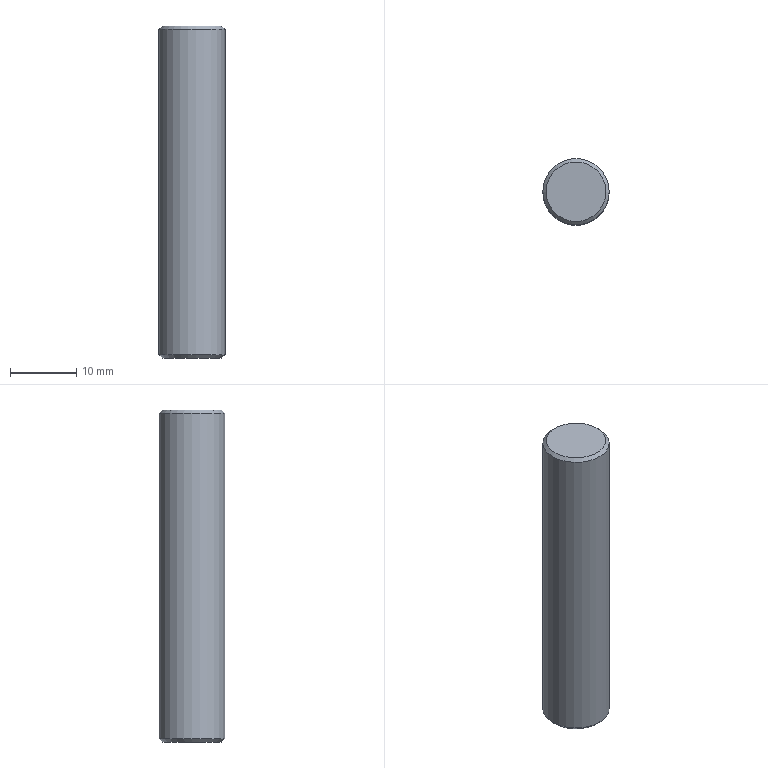Part | STEP file | D8-50_id50_x_t | 1 solid | 5 faces | box 10 x 10 x 50 mm | volume 3919 mm3 | plane 2 | cone 2 | cylinder 1 | commonest cylinder face diameters 10 x1
STEP:
#1=CARTESIAN_POINT('',(-224.05,-48.,-64.5));
#2=VERTEX_POINT('',#1);
#3=CARTESIAN_POINT('',(-219.55,-48.,-64.5));
#4=DIRECTION('',(0.,0.,-1.));
#5=DIRECTION('',(-1.,0.,0.));
#6=AXIS2_PLACEMENT_3D('',#3,#4,#5);
#7=CIRCLE('',#6,4.5);
#8=EDGE_CURVE('',#2,#2,#7,.T.);
#9=ORIENTED_EDGE('',*,*,#8,.T.);
#10=EDGE_LOOP('',(#9));
#11=FACE_OUTER_BOUND('',#10,.T.);
#12=CARTESIAN_POINT('',(-219.55,-48.,-64.5));
#13=DIRECTION('',(0.,0.,-1.));
#14=DIRECTION('',(-1.,0.,0.));
#15=AXIS2_PLACEMENT_3D('',#12,#13,#14);
#16=PLANE('',#15);
#17=ADVANCED_FACE('',(#11),#16,.T.);
#18=CARTESIAN_POINT('',(-224.55,-48.,-64.));
#19=VERTEX_POINT('',#18);
#20=CARTESIAN_POINT('',(-219.55,-48.,-64.));
#21=DIRECTION('',(0.,0.,1.));
#22=DIRECTION('',(-1.,0.,0.));
#23=AXIS2_PLACEMENT_3D('',#20,#21,#22);
#24=CIRCLE('',#23,5.);
#25=EDGE_CURVE('',#19,#19,#24,.T.);
#26=ORIENTED_EDGE('',*,*,#25,.T.);
#27=EDGE_LOOP('',(#26));
#28=FACE_BOUND('',#27,.T.);
#29=CARTESIAN_POINT('',(-214.55,-48.,-15.));
#30=VERTEX_POINT('',#29);
#31=CARTESIAN_POINT('',(-219.55,-48.,-15.));
#32=DIRECTION('',(0.,0.,-1.));
#33=DIRECTION('',(1.,0.,0.));
#34=AXIS2_PLACEMENT_3D('',#31,#32,#33);
#35=CIRCLE('',#34,5.);
#36=EDGE_CURVE('',#30,#30,#35,.T.);
#37=ORIENTED_EDGE('',*,*,#36,.T.);
#38=EDGE_LOOP('',(#37));
#39=FACE_BOUND('',#38,.T.);
#40=CARTESIAN_POINT('',(-219.55,-48.,-47.));
#41=DIRECTION('',(0.,0.,-1.));
#42=DIRECTION('',(1.,0.,0.));
#43=AXIS2_PLACEMENT_3D('',#40,#41,#42);
#44=CYLINDRICAL_SURFACE('',#43,5.);
#45=ADVANCED_FACE('',(#28,#39),#44,.T.);
#46=CARTESIAN_POINT('',(-215.05,-48.,-14.5));
#47=VERTEX_POINT('',#46);
#48=CARTESIAN_POINT('',(-219.55,-48.,-14.5));
#49=DIRECTION('',(0.,0.,1.));
#50=DIRECTION('',(1.,0.,0.));
#51=AXIS2_PLACEMENT_3D('',#48,#49,#50);
#52=CIRCLE('',#51,4.5);
#53=EDGE_CURVE('',#47,#47,#52,.T.);
#54=ORIENTED_EDGE('',*,*,#53,.T.);
#55=EDGE_LOOP('',(#54));
#56=FACE_OUTER_BOUND('',#55,.T.);
#57=CARTESIAN_POINT('',(-219.55,-48.,-14.5));
#58=DIRECTION('',(0.,0.,1.));
#59=DIRECTION('',(1.,0.,0.));
#60=AXIS2_PLACEMENT_3D('',#57,#58,#59);
#61=PLANE('',#60);
#62=ADVANCED_FACE('',(#56),#61,.T.);
#63=ORIENTED_EDGE('',*,*,#8,.F.);
#64=EDGE_LOOP('',(#63));
#65=FACE_BOUND('',#64,.T.);
#66=ORIENTED_EDGE('',*,*,#25,.F.);
#67=EDGE_LOOP('',(#66));
#68=FACE_BOUND('',#67,.T.);
#69=CARTESIAN_POINT('',(-219.55,-48.,-64.));
#70=DIRECTION('',(0.,0.,1.));
#71=DIRECTION('',(1.,0.,0.));
#72=AXIS2_PLACEMENT_3D('',#69,#70,#71);
#73=CONICAL_SURFACE('',#72,5.,45.);
#74=ADVANCED_FACE('',(#65,#68),#73,.T.);
#75=ORIENTED_EDGE('',*,*,#53,.F.);
#76=EDGE_LOOP('',(#75));
#77=FACE_BOUND('',#76,.T.);
#78=ORIENTED_EDGE('',*,*,#36,.F.);
#79=EDGE_LOOP('',(#78));
#80=FACE_BOUND('',#79,.T.);
#81=CARTESIAN_POINT('',(-219.55,-48.,-15.));
#82=DIRECTION('',(0.,0.,-1.));
#83=DIRECTION('',(-1.,0.,0.));
#84=AXIS2_PLACEMENT_3D('',#81,#82,#83);
#85=CONICAL_SURFACE('',#84,5.,45.);
#86=ADVANCED_FACE('',(#77,#80),#85,.T.);
#87=CLOSED_SHELL('',(#17,#45,#62,#74,#86));
#88=MANIFOLD_SOLID_BREP('',#87);
#89=(LENGTH_UNIT()NAMED_UNIT(*)SI_UNIT(.MILLI.,.METRE.));
#90=UNCERTAINTY_MEASURE_WITH_UNIT(LENGTH_MEASURE(0.00002),#89,'','');
#91=(NAMED_UNIT(*)PLANE_ANGLE_UNIT()SI_UNIT($,.RADIAN.));
#92=PLANE_ANGLE_MEASURE_WITH_UNIT(PLANE_ANGLE_MEASURE(0.01745),#91);
#93=DIMENSIONAL_EXPONENTS(0.,0.,0.,0.,0.,0.,0.);
#94=(CONVERSION_BASED_UNIT('DEGREE',#92)NAMED_UNIT(#93)PLANE_ANGLE_UNIT());
#95=(NAMED_UNIT(*)SI_UNIT($,.STERADIAN.)SOLID_ANGLE_UNIT());
#96=(GEOMETRIC_REPRESENTATION_CONTEXT(3)GLOBAL_UNCERTAINTY_ASSIGNED_CONTEXT((#90))GLOBAL_UNIT_ASSIGNED_CONTEXT((#89,#94,#95))REPRESENTATION_CONTEXT('',''));
#97=ADVANCED_BREP_SHAPE_REPRESENTATION('',(#88),#96);